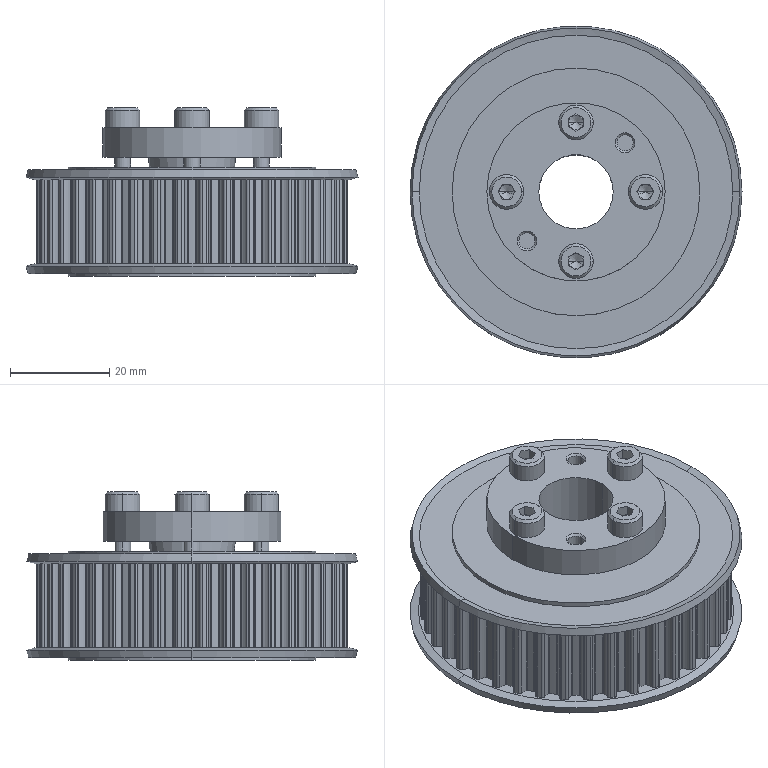Part | STEP file | 001-010-ECC15-S5M150-40-E-d15 | 1 solid | 485 faces | box 67 x 67 x 34 mm | volume 65778 mm3 | cylinder 385 | plane 60 | cone 40 | commonest cylinder face diameters 1.1 x98 0.5 x92 6.55 x86 59.16 x41 62.7 x40 3.242 x12